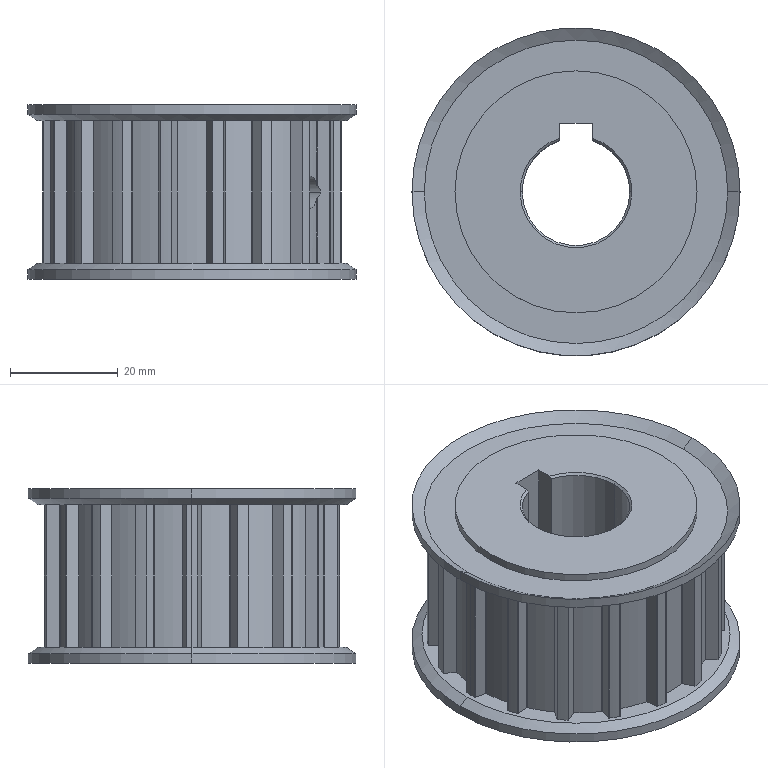Part | SolidWorks | features ICE 10, Chamfer 9, RevCut 3, CirPattern 2, Revolution 2 | 1 solid | 203 faces | box 61 x 61 x 32.5 mm | volume 59006 mm3 | cylinder 143 | plane 46 | cone 14 | commonest cylinder face diameters 0.2 x89 50.73 x20 55.45 x19 6 x4 45 x4 61 x4